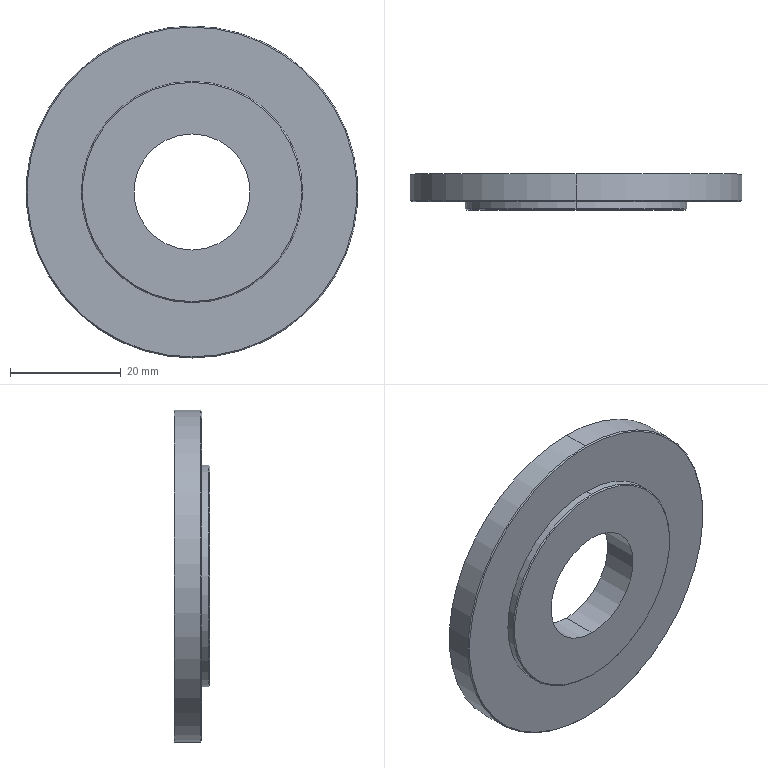Part | STEP file | Guide wheel mechanism revised.sldasm-Part-432 | 1 solid | 25 faces | box 60 x 6.5 x 60 mm | volume 13262 mm3 | cylinder 14 | plane 7 | cone 4 | commonest cylinder face diameters 8 x8 21 x2 40 x2 60 x2
STEP:
#1=CARTESIAN_POINT('',(0.,-1.5,-19.8));
#2=VERTEX_POINT('',#1);
#3=CARTESIAN_POINT('',(0.,-1.5,19.8));
#4=VERTEX_POINT('',#3);
#5=CARTESIAN_POINT('',(0.,-1.5,0.));
#6=DIRECTION('',(0.,-1.,0.));
#7=DIRECTION('',(0.,0.,1.));
#8=AXIS2_PLACEMENT_3D('',#5,#6,#7);
#9=CIRCLE('',#8,19.8);
#10=EDGE_CURVE('',#2,#4,#9,.T.);
#11=ORIENTED_EDGE('',*,*,#10,.F.);
#12=CARTESIAN_POINT('',(0.,-1.3,-20.));
#13=VERTEX_POINT('',#12);
#14=CARTESIAN_POINT('',(0.,-1.3,-20.));
#15=DIRECTION('',(0.,0.7071,-0.7071));
#16=VECTOR('',#15,1000.);
#17=LINE('',#14,#16);
#18=EDGE_CURVE('',#2,#13,#17,.T.);
#19=ORIENTED_EDGE('',*,*,#18,.T.);
#20=CARTESIAN_POINT('',(0.,-1.3,20.));
#21=VERTEX_POINT('',#20);
#22=CARTESIAN_POINT('',(0.,-1.3,0.));
#23=DIRECTION('',(0.,1.,0.));
#24=DIRECTION('',(0.,0.,1.));
#25=AXIS2_PLACEMENT_3D('',#22,#23,#24);
#26=CIRCLE('',#25,20.);
#27=EDGE_CURVE('',#21,#13,#26,.T.);
#28=ORIENTED_EDGE('',*,*,#27,.F.);
#29=CARTESIAN_POINT('',(0.,-1.3,20.));
#30=DIRECTION('',(0.,0.7071,0.7071));
#31=VECTOR('',#30,1000.);
#32=LINE('',#29,#31);
#33=EDGE_CURVE('',#4,#21,#32,.T.);
#34=ORIENTED_EDGE('',*,*,#33,.F.);
#35=EDGE_LOOP('',(#11,#19,#28,#34));
#36=FACE_OUTER_BOUND('',#35,.T.);
#37=CARTESIAN_POINT('',(0.,-1.3,0.));
#38=DIRECTION('',(0.,1.,0.));
#39=DIRECTION('',(0.,0.,1.));
#40=AXIS2_PLACEMENT_3D('',#37,#38,#39);
#41=CONICAL_SURFACE('',#40,20.,0.7854);
#42=ADVANCED_FACE('',(#36),#41,.T.);
#43=CARTESIAN_POINT('',(0.,0.,-29.8));
#44=VERTEX_POINT('',#43);
#45=CARTESIAN_POINT('',(0.,0.,29.8));
#46=VERTEX_POINT('',#45);
#47=CARTESIAN_POINT('',(0.,0.,0.));
#48=DIRECTION('',(0.,-1.,0.));
#49=DIRECTION('',(0.,0.,1.));
#50=AXIS2_PLACEMENT_3D('',#47,#48,#49);
#51=CIRCLE('',#50,29.8);
#52=EDGE_CURVE('',#44,#46,#51,.T.);
#53=ORIENTED_EDGE('',*,*,#52,.F.);
#54=CARTESIAN_POINT('',(0.,0.2,-30.));
#55=VERTEX_POINT('',#54);
#56=CARTESIAN_POINT('',(0.,0.2,-30.));
#57=DIRECTION('',(0.,0.7071,-0.7071));
#58=VECTOR('',#57,1000.);
#59=LINE('',#56,#58);
#60=EDGE_CURVE('',#44,#55,#59,.T.);
#61=ORIENTED_EDGE('',*,*,#60,.T.);
#62=CARTESIAN_POINT('',(0.,0.2,30.));
#63=VERTEX_POINT('',#62);
#64=CARTESIAN_POINT('',(0.,0.2,0.));
#65=DIRECTION('',(0.,1.,0.));
#66=DIRECTION('',(0.,0.,1.));
#67=AXIS2_PLACEMENT_3D('',#64,#65,#66);
#68=CIRCLE('',#67,30.);
#69=EDGE_CURVE('',#63,#55,#68,.T.);
#70=ORIENTED_EDGE('',*,*,#69,.F.);
#71=CARTESIAN_POINT('',(0.,0.2,30.));
#72=DIRECTION('',(0.,0.7071,0.7071));
#73=VECTOR('',#72,1000.);
#74=LINE('',#71,#73);
#75=EDGE_CURVE('',#46,#63,#74,.T.);
#76=ORIENTED_EDGE('',*,*,#75,.F.);
#77=EDGE_LOOP('',(#53,#61,#70,#76));
#78=FACE_OUTER_BOUND('',#77,.T.);
#79=CARTESIAN_POINT('',(0.,0.2,0.));
#80=DIRECTION('',(0.,1.,0.));
#81=DIRECTION('',(0.,0.,1.));
#82=AXIS2_PLACEMENT_3D('',#79,#80,#81);
#83=CONICAL_SURFACE('',#82,30.,0.7854);
#84=ADVANCED_FACE('',(#78),#83,.T.);
#85=ORIENTED_EDGE('',*,*,#27,.T.);
#86=CARTESIAN_POINT('',(0.,0.,-20.));
#87=VERTEX_POINT('',#86);
#88=CARTESIAN_POINT('',(0.,-1.5,-20.));
#89=DIRECTION('',(0.,1.,0.));
#90=VECTOR('',#89,1000.);
#91=LINE('',#88,#90);
#92=EDGE_CURVE('',#13,#87,#91,.T.);
#93=ORIENTED_EDGE('',*,*,#92,.T.);
#94=CARTESIAN_POINT('',(0.,0.,20.));
#95=VERTEX_POINT('',#94);
#96=CARTESIAN_POINT('',(0.,0.,0.));
#97=DIRECTION('',(0.,1.,0.));
#98=DIRECTION('',(0.,0.,1.));
#99=AXIS2_PLACEMENT_3D('',#96,#97,#98);
#100=CIRCLE('',#99,20.);
#101=EDGE_CURVE('',#95,#87,#100,.T.);
#102=ORIENTED_EDGE('',*,*,#101,.F.);
#103=CARTESIAN_POINT('',(0.,-1.5,20.));
#104=DIRECTION('',(0.,1.,0.));
#105=VECTOR('',#104,1000.);
#106=LINE('',#103,#105);
#107=EDGE_CURVE('',#21,#95,#106,.T.);
#108=ORIENTED_EDGE('',*,*,#107,.F.);
#109=EDGE_LOOP('',(#85,#93,#102,#108));
#110=FACE_OUTER_BOUND('',#109,.T.);
#111=CARTESIAN_POINT('',(0.,-1.5,0.));
#112=DIRECTION('',(0.,1.,0.));
#113=DIRECTION('',(0.,0.,1.));
#114=AXIS2_PLACEMENT_3D('',#111,#112,#113);
#115=CYLINDRICAL_SURFACE('',#114,20.);
#116=ADVANCED_FACE('',(#110),#115,.T.);
#117=CARTESIAN_POINT('',(0.,2.5,16.));
#118=VERTEX_POINT('',#117);
#119=CARTESIAN_POINT('',(0.,2.5,24.));
#120=VERTEX_POINT('',#119);
#121=CARTESIAN_POINT('',(0.,2.5,20.));
#122=DIRECTION('',(0.,1.,0.));
#123=DIRECTION('',(0.,0.,1.));
#124=AXIS2_PLACEMENT_3D('',#121,#122,#123);
#125=CIRCLE('',#124,4.);
#126=EDGE_CURVE('',#118,#120,#125,.T.);
#127=ORIENTED_EDGE('',*,*,#126,.F.);
#128=CARTESIAN_POINT('',(0.,5.,16.));
#129=VERTEX_POINT('',#128);
#130=CARTESIAN_POINT('',(0.,2.5,16.));
#131=DIRECTION('',(0.,1.,0.));
#132=VECTOR('',#131,1000.);
#133=LINE('',#130,#132);
#134=EDGE_CURVE('',#118,#129,#133,.T.);
#135=ORIENTED_EDGE('',*,*,#134,.T.);
#136=CARTESIAN_POINT('',(0.,5.,24.));
#137=VERTEX_POINT('',#136);
#138=CARTESIAN_POINT('',(0.,5.,20.));
#139=DIRECTION('',(0.,1.,0.));
#140=DIRECTION('',(0.,0.,1.));
#141=AXIS2_PLACEMENT_3D('',#138,#139,#140);
#142=CIRCLE('',#141,4.);
#143=EDGE_CURVE('',#129,#137,#142,.T.);
#144=ORIENTED_EDGE('',*,*,#143,.T.);
#145=CARTESIAN_POINT('',(0.,2.5,24.));
#146=DIRECTION('',(0.,1.,0.));
#147=VECTOR('',#146,1000.);
#148=LINE('',#145,#147);
#149=EDGE_CURVE('',#120,#137,#148,.T.);
#150=ORIENTED_EDGE('',*,*,#149,.F.);
#151=EDGE_LOOP('',(#127,#135,#144,#150));
#152=FACE_OUTER_BOUND('',#151,.T.);
#153=CARTESIAN_POINT('',(0.,2.5,20.));
#154=DIRECTION('',(0.,1.,0.));
#155=DIRECTION('',(0.,0.,1.));
#156=AXIS2_PLACEMENT_3D('',#153,#154,#155);
#157=CYLINDRICAL_SURFACE('',#156,4.);
#158=ADVANCED_FACE('',(#152),#157,.F.);
#159=CARTESIAN_POINT('',(20.,2.5,-4.));
#160=VERTEX_POINT('',#159);
#161=CARTESIAN_POINT('',(20.,2.5,4.));
#162=VERTEX_POINT('',#161);
#163=CARTESIAN_POINT('',(20.,2.5,0.));
#164=DIRECTION('',(0.,1.,0.));
#165=DIRECTION('',(0.,0.,1.));
#166=AXIS2_PLACEMENT_3D('',#163,#164,#165);
#167=CIRCLE('',#166,4.);
#168=EDGE_CURVE('',#160,#162,#167,.T.);
#169=ORIENTED_EDGE('',*,*,#168,.F.);
#170=CARTESIAN_POINT('',(20.,5.,-4.));
#171=VERTEX_POINT('',#170);
#172=CARTESIAN_POINT('',(20.,2.5,-4.));
#173=DIRECTION('',(0.,1.,0.));
#174=VECTOR('',#173,1000.);
#175=LINE('',#172,#174);
#176=EDGE_CURVE('',#160,#171,#175,.T.);
#177=ORIENTED_EDGE('',*,*,#176,.T.);
#178=CARTESIAN_POINT('',(20.,5.,4.));
#179=VERTEX_POINT('',#178);
#180=CARTESIAN_POINT('',(20.,5.,0.));
#181=DIRECTION('',(0.,1.,0.));
#182=DIRECTION('',(0.,0.,1.));
#183=AXIS2_PLACEMENT_3D('',#180,#181,#182);
#184=CIRCLE('',#183,4.);
#185=EDGE_CURVE('',#171,#179,#184,.T.);
#186=ORIENTED_EDGE('',*,*,#185,.T.);
#187=CARTESIAN_POINT('',(20.,2.5,4.));
#188=DIRECTION('',(0.,1.,0.));
#189=VECTOR('',#188,1000.);
#190=LINE('',#187,#189);
#191=EDGE_CURVE('',#162,#179,#190,.T.);
#192=ORIENTED_EDGE('',*,*,#191,.F.);
#193=EDGE_LOOP('',(#169,#177,#186,#192));
#194=FACE_OUTER_BOUND('',#193,.T.);
#195=CARTESIAN_POINT('',(20.,2.5,0.));
#196=DIRECTION('',(0.,1.,0.));
#197=DIRECTION('',(0.,0.,1.));
#198=AXIS2_PLACEMENT_3D('',#195,#196,#197);
#199=CYLINDRICAL_SURFACE('',#198,4.);
#200=ADVANCED_FACE('',(#194),#199,.F.);
#201=CARTESIAN_POINT('',(-20.,2.5,-4.));
#202=VERTEX_POINT('',#201);
#203=CARTESIAN_POINT('',(-20.,2.5,4.));
#204=VERTEX_POINT('',#203);
#205=CARTESIAN_POINT('',(-20.,2.5,0.));
#206=DIRECTION('',(0.,1.,0.));
#207=DIRECTION('',(0.,0.,1.));
#208=AXIS2_PLACEMENT_3D('',#205,#206,#207);
#209=CIRCLE('',#208,4.);
#210=EDGE_CURVE('',#202,#204,#209,.T.);
#211=ORIENTED_EDGE('',*,*,#210,.F.);
#212=CARTESIAN_POINT('',(-20.,5.,-4.));
#213=VERTEX_POINT('',#212);
#214=CARTESIAN_POINT('',(-20.,2.5,-4.));
#215=DIRECTION('',(0.,1.,0.));
#216=VECTOR('',#215,1000.);
#217=LINE('',#214,#216);
#218=EDGE_CURVE('',#202,#213,#217,.T.);
#219=ORIENTED_EDGE('',*,*,#218,.T.);
#220=CARTESIAN_POINT('',(-20.,5.,4.));
#221=VERTEX_POINT('',#220);
#222=CARTESIAN_POINT('',(-20.,5.,0.));
#223=DIRECTION('',(0.,1.,0.));
#224=DIRECTION('',(0.,0.,1.));
#225=AXIS2_PLACEMENT_3D('',#222,#223,#224);
#226=CIRCLE('',#225,4.);
#227=EDGE_CURVE('',#213,#221,#226,.T.);
#228=ORIENTED_EDGE('',*,*,#227,.T.);
#229=CARTESIAN_POINT('',(-20.,2.5,4.));
#230=DIRECTION('',(0.,1.,0.));
#231=VECTOR('',#230,1000.);
#232=LINE('',#229,#231);
#233=EDGE_CURVE('',#204,#221,#232,.T.);
#234=ORIENTED_EDGE('',*,*,#233,.F.);
#235=EDGE_LOOP('',(#211,#219,#228,#234));
#236=FACE_OUTER_BOUND('',#235,.T.);
#237=CARTESIAN_POINT('',(-20.,2.5,0.));
#238=DIRECTION('',(0.,1.,0.));
#239=DIRECTION('',(0.,0.,1.));
#240=AXIS2_PLACEMENT_3D('',#237,#238,#239);
#241=CYLINDRICAL_SURFACE('',#240,4.);
#242=ADVANCED_FACE('',(#236),#241,.F.);
#243=CARTESIAN_POINT('',(0.,2.5,-24.));
#244=VERTEX_POINT('',#243);
#245=CARTESIAN_POINT('',(0.,2.5,-16.));
#246=VERTEX_POINT('',#245);
#247=CARTESIAN_POINT('',(0.,2.5,-20.));
#248=DIRECTION('',(0.,1.,0.));
#249=DIRECTION('',(0.,0.,1.));
#250=AXIS2_PLACEMENT_3D('',#247,#248,#249);
#251=CIRCLE('',#250,4.);
#252=EDGE_CURVE('',#244,#246,#251,.T.);
#253=ORIENTED_EDGE('',*,*,#252,.F.);
#254=CARTESIAN_POINT('',(0.,5.,-24.));
#255=VERTEX_POINT('',#254);
#256=CARTESIAN_POINT('',(0.,2.5,-24.));
#257=DIRECTION('',(0.,1.,0.));
#258=VECTOR('',#257,1000.);
#259=LINE('',#256,#258);
#260=EDGE_CURVE('',#244,#255,#259,.T.);
#261=ORIENTED_EDGE('',*,*,#260,.T.);
#262=CARTESIAN_POINT('',(0.,5.,-16.));
#263=VERTEX_POINT('',#262);
#264=CARTESIAN_POINT('',(0.,5.,-20.));
#265=DIRECTION('',(0.,1.,0.));
#266=DIRECTION('',(0.,0.,1.));
#267=AXIS2_PLACEMENT_3D('',#264,#265,#266);
#268=CIRCLE('',#267,4.);
#269=EDGE_CURVE('',#255,#263,#268,.T.);
#270=ORIENTED_EDGE('',*,*,#269,.T.);
#271=CARTESIAN_POINT('',(0.,2.5,-16.));
#272=DIRECTION('',(0.,1.,0.));
#273=VECTOR('',#272,1000.);
#274=LINE('',#271,#273);
#275=EDGE_CURVE('',#246,#263,#274,.T.);
#276=ORIENTED_EDGE('',*,*,#275,.F.);
#277=EDGE_LOOP('',(#253,#261,#270,#276));
#278=FACE_OUTER_BOUND('',#277,.T.);
#279=CARTESIAN_POINT('',(0.,2.5,-20.));
#280=DIRECTION('',(0.,1.,0.));
#281=DIRECTION('',(0.,0.,1.));
#282=AXIS2_PLACEMENT_3D('',#279,#280,#281);
#283=CYLINDRICAL_SURFACE('',#282,4.);
#284=ADVANCED_FACE('',(#278),#283,.F.);
#285=CARTESIAN_POINT('',(0.,5.,-10.5));
#286=VERTEX_POINT('',#285);
#287=CARTESIAN_POINT('',(0.,5.,10.5));
#288=VERTEX_POINT('',#287);
#289=CARTESIAN_POINT('',(0.,5.,0.));
#290=DIRECTION('',(0.,1.,0.));
#291=DIRECTION('',(0.,0.,1.));
#292=AXIS2_PLACEMENT_3D('',#289,#290,#291);
#293=CIRCLE('',#292,10.5);
#294=EDGE_CURVE('',#286,#288,#293,.T.);
#295=ORIENTED_EDGE('',*,*,#294,.T.);
#296=CARTESIAN_POINT('',(0.,-1.5,10.5));
#297=VERTEX_POINT('',#296);
#298=CARTESIAN_POINT('',(0.,5.,10.5));
#299=DIRECTION('',(0.,-1.,0.));
#300=VECTOR('',#299,1000.);
#301=LINE('',#298,#300);
#302=EDGE_CURVE('',#288,#297,#301,.T.);
#303=ORIENTED_EDGE('',*,*,#302,.T.);
#304=CARTESIAN_POINT('',(0.,-1.5,-10.5));
#305=VERTEX_POINT('',#304);
#306=CARTESIAN_POINT('',(0.,-1.5,0.));
#307=DIRECTION('',(0.,1.,0.));
#308=DIRECTION('',(0.,0.,1.));
#309=AXIS2_PLACEMENT_3D('',#306,#307,#308);
#310=CIRCLE('',#309,10.5);
#311=EDGE_CURVE('',#305,#297,#310,.T.);
#312=ORIENTED_EDGE('',*,*,#311,.F.);
#313=CARTESIAN_POINT('',(0.,5.,-10.5));
#314=DIRECTION('',(0.,-1.,0.));
#315=VECTOR('',#314,1000.);
#316=LINE('',#313,#315);
#317=EDGE_CURVE('',#286,#305,#316,.T.);
#318=ORIENTED_EDGE('',*,*,#317,.F.);
#319=EDGE_LOOP('',(#295,#303,#312,#318));
#320=FACE_OUTER_BOUND('',#319,.T.);
#321=CARTESIAN_POINT('',(0.,5.,0.));
#322=DIRECTION('',(0.,-1.,0.));
#323=DIRECTION('',(0.,0.,-1.));
#324=AXIS2_PLACEMENT_3D('',#321,#322,#323);
#325=CYLINDRICAL_SURFACE('',#324,10.5);
#326=ADVANCED_FACE('',(#320),#325,.F.);
#327=CARTESIAN_POINT('',(0.,5.,30.));
#328=VERTEX_POINT('',#327);
#329=CARTESIAN_POINT('',(0.,5.,-30.));
#330=VERTEX_POINT('',#329);
#331=CARTESIAN_POINT('',(0.,5.,0.));
#332=DIRECTION('',(0.,1.,0.));
#333=DIRECTION('',(0.,0.,1.));
#334=AXIS2_PLACEMENT_3D('',#331,#332,#333);
#335=CIRCLE('',#334,30.);
#336=EDGE_CURVE('',#328,#330,#335,.T.);
#337=ORIENTED_EDGE('',*,*,#336,.F.);
#338=CARTESIAN_POINT('',(0.,5.,30.));
#339=DIRECTION('',(0.,-1.,0.));
#340=VECTOR('',#339,1000.);
#341=LINE('',#338,#340);
#342=EDGE_CURVE('',#328,#63,#341,.T.);
#343=ORIENTED_EDGE('',*,*,#342,.T.);
#344=ORIENTED_EDGE('',*,*,#69,.T.);
#345=CARTESIAN_POINT('',(0.,5.,-30.));
#346=DIRECTION('',(0.,-1.,0.));
#347=VECTOR('',#346,1000.);
#348=LINE('',#345,#347);
#349=EDGE_CURVE('',#330,#55,#348,.T.);
#350=ORIENTED_EDGE('',*,*,#349,.F.);
#351=EDGE_LOOP('',(#337,#343,#344,#350));
#352=FACE_OUTER_BOUND('',#351,.T.);
#353=CARTESIAN_POINT('',(0.,5.,0.));
#354=DIRECTION('',(0.,-1.,0.));
#355=DIRECTION('',(0.,0.,-1.));
#356=AXIS2_PLACEMENT_3D('',#353,#354,#355);
#357=CYLINDRICAL_SURFACE('',#356,30.);
#358=ADVANCED_FACE('',(#352),#357,.T.);
#359=CARTESIAN_POINT('',(0.,5.,20.));
#360=DIRECTION('',(0.,1.,0.));
#361=DIRECTION('',(0.,0.,1.));
#362=AXIS2_PLACEMENT_3D('',#359,#360,#361);
#363=CIRCLE('',#362,4.);
#364=EDGE_CURVE('',#137,#129,#363,.T.);
#365=ORIENTED_EDGE('',*,*,#364,.F.);
#366=ORIENTED_EDGE('',*,*,#143,.F.);
#367=EDGE_LOOP('',(#365,#366));
#368=FACE_BOUND('',#367,.T.);
#369=CARTESIAN_POINT('',(20.,5.,0.));
#370=DIRECTION('',(0.,1.,0.));
#371=DIRECTION('',(0.,0.,1.));
#372=AXIS2_PLACEMENT_3D('',#369,#370,#371);
#373=CIRCLE('',#372,4.);
#374=EDGE_CURVE('',#179,#171,#373,.T.);
#375=ORIENTED_EDGE('',*,*,#374,.F.);
#376=ORIENTED_EDGE('',*,*,#185,.F.);
#377=EDGE_LOOP('',(#375,#376));
#378=FACE_BOUND('',#377,.T.);
#379=CARTESIAN_POINT('',(-20.,5.,0.));
#380=DIRECTION('',(0.,1.,0.));
#381=DIRECTION('',(0.,0.,1.));
#382=AXIS2_PLACEMENT_3D('',#379,#380,#381);
#383=CIRCLE('',#382,4.);
#384=EDGE_CURVE('',#221,#213,#383,.T.);
#385=ORIENTED_EDGE('',*,*,#384,.F.);
#386=ORIENTED_EDGE('',*,*,#227,.F.);
#387=EDGE_LOOP('',(#385,#386));
#388=FACE_BOUND('',#387,.T.);
#389=CARTESIAN_POINT('',(0.,5.,-20.));
#390=DIRECTION('',(0.,1.,0.));
#391=DIRECTION('',(0.,0.,1.));
#392=AXIS2_PLACEMENT_3D('',#389,#390,#391);
#393=CIRCLE('',#392,4.);
#394=EDGE_CURVE('',#263,#255,#393,.T.);
#395=ORIENTED_EDGE('',*,*,#394,.F.);
#396=ORIENTED_EDGE('',*,*,#269,.F.);
#397=EDGE_LOOP('',(#395,#396));
#398=FACE_BOUND('',#397,.T.);
#399=CARTESIAN_POINT('',(0.,5.,0.));
#400=DIRECTION('',(0.,1.,0.));
#401=DIRECTION('',(0.,0.,1.));
#402=AXIS2_PLACEMENT_3D('',#399,#400,#401);
#403=CIRCLE('',#402,30.);
#404=EDGE_CURVE('',#330,#328,#403,.T.);
#405=ORIENTED_EDGE('',*,*,#404,.T.);
#406=ORIENTED_EDGE('',*,*,#336,.T.);
#407=EDGE_LOOP('',(#405,#406));
#408=FACE_OUTER_BOUND('',#407,.T.);
#409=ORIENTED_EDGE('',*,*,#294,.F.);
#410=CARTESIAN_POINT('',(0.,5.,0.));
#411=DIRECTION('',(0.,1.,0.));
#412=DIRECTION('',(0.,0.,1.));
#413=AXIS2_PLACEMENT_3D('',#410,#411,#412);
#414=CIRCLE('',#413,10.5);
#415=EDGE_CURVE('',#288,#286,#414,.T.);
#416=ORIENTED_EDGE('',*,*,#415,.F.);
#417=EDGE_LOOP('',(#409,#416));
#418=FACE_BOUND('',#417,.T.);
#419=CARTESIAN_POINT('',(0.,5.,0.));
#420=DIRECTION('',(0.,1.,0.));
#421=DIRECTION('',(0.,0.,1.));
#422=AXIS2_PLACEMENT_3D('',#419,#420,#421);
#423=PLANE('',#422);
#424=ADVANCED_FACE('',(#368,#378,#388,#398,#408,#418),#423,.T.);
#425=CARTESIAN_POINT('',(0.,0.,0.));
#426=DIRECTION('',(0.,-1.,0.));
#427=DIRECTION('',(0.,0.,1.));
#428=AXIS2_PLACEMENT_3D('',#425,#426,#427);
#429=CIRCLE('',#428,29.8);
#430=EDGE_CURVE('',#46,#44,#429,.T.);
#431=ORIENTED_EDGE('',*,*,#430,.T.);
#432=ORIENTED_EDGE('',*,*,#52,.T.);
#433=EDGE_LOOP('',(#431,#432));
#434=FACE_OUTER_BOUND('',#433,.T.);
#435=ORIENTED_EDGE('',*,*,#101,.T.);
#436=CARTESIAN_POINT('',(0.,0.,0.));
#437=DIRECTION('',(0.,1.,0.));
#438=DIRECTION('',(0.,0.,1.));
#439=AXIS2_PLACEMENT_3D('',#436,#437,#438);
#440=CIRCLE('',#439,20.);
#441=EDGE_CURVE('',#87,#95,#440,.T.);
#442=ORIENTED_EDGE('',*,*,#441,.T.);
#443=EDGE_LOOP('',(#435,#442));
#444=FACE_BOUND('',#443,.T.);
#445=CARTESIAN_POINT('',(0.,0.,0.));
#446=DIRECTION('',(0.,1.,0.));
#447=DIRECTION('',(0.,0.,1.));
#448=AXIS2_PLACEMENT_3D('',#445,#446,#447);
#449=PLANE('',#448);
#450=ADVANCED_FACE('',(#434,#444),#449,.F.);
#451=ORIENTED_EDGE('',*,*,#342,.F.);
#452=ORIENTED_EDGE('',*,*,#404,.F.);
#453=ORIENTED_EDGE('',*,*,#349,.T.);
#454=CARTESIAN_POINT('',(0.,0.2,0.));
#455=DIRECTION('',(0.,1.,0.));
#456=DIRECTION('',(0.,0.,1.));
#457=AXIS2_PLACEMENT_3D('',#454,#455,#456);
#458=CIRCLE('',#457,30.);
#459=EDGE_CURVE('',#55,#63,#458,.T.);
#460=ORIENTED_EDGE('',*,*,#459,.T.);
#461=EDGE_LOOP('',(#451,#452,#453,#460));
#462=FACE_OUTER_BOUND('',#461,.T.);
#463=CARTESIAN_POINT('',(0.,5.,0.));
#464=DIRECTION('',(0.,-1.,0.));
#465=DIRECTION('',(0.,0.,-1.));
#466=AXIS2_PLACEMENT_3D('',#463,#464,#465);
#467=CYLINDRICAL_SURFACE('',#466,30.);
#468=ADVANCED_FACE('',(#462),#467,.T.);
#469=ORIENTED_EDGE('',*,*,#302,.F.);
#470=ORIENTED_EDGE('',*,*,#415,.T.);
#471=ORIENTED_EDGE('',*,*,#317,.T.);
#472=CARTESIAN_POINT('',(0.,-1.5,0.));
#473=DIRECTION('',(0.,1.,0.));
#474=DIRECTION('',(0.,0.,1.));
#475=AXIS2_PLACEMENT_3D('',#472,#473,#474);
#476=CIRCLE('',#475,10.5);
#477=EDGE_CURVE('',#297,#305,#476,.T.);
#478=ORIENTED_EDGE('',*,*,#477,.F.);
#479=EDGE_LOOP('',(#469,#470,#471,#478));
#480=FACE_OUTER_BOUND('',#479,.T.);
#481=CARTESIAN_POINT('',(0.,5.,0.));
#482=DIRECTION('',(0.,-1.,0.));
#483=DIRECTION('',(0.,0.,-1.));
#484=AXIS2_PLACEMENT_3D('',#481,#482,#483);
#485=CYLINDRICAL_SURFACE('',#484,10.5);
#486=ADVANCED_FACE('',(#480),#485,.F.);
#487=ORIENTED_EDGE('',*,*,#260,.F.);
#488=CARTESIAN_POINT('',(0.,2.5,-20.));
#489=DIRECTION('',(0.,1.,0.));
#490=DIRECTION('',(0.,0.,1.));
#491=AXIS2_PLACEMENT_3D('',#488,#489,#490);
#492=CIRCLE('',#491,4.);
#493=EDGE_CURVE('',#246,#244,#492,.T.);
#494=ORIENTED_EDGE('',*,*,#493,.F.);
#495=ORIENTED_EDGE('',*,*,#275,.T.);
#496=ORIENTED_EDGE('',*,*,#394,.T.);
#497=EDGE_LOOP('',(#487,#494,#495,#496));
#498=FACE_OUTER_BOUND('',#497,.T.);
#499=CARTESIAN_POINT('',(0.,2.5,-20.));
#500=DIRECTION('',(0.,1.,0.));
#501=DIRECTION('',(0.,0.,1.));
#502=AXIS2_PLACEMENT_3D('',#499,#500,#501);
#503=CYLINDRICAL_SURFACE('',#502,4.);
#504=ADVANCED_FACE('',(#498),#503,.F.);
#505=ORIENTED_EDGE('',*,*,#493,.T.);
#506=ORIENTED_EDGE('',*,*,#252,.T.);
#507=EDGE_LOOP('',(#505,#506));
#508=FACE_OUTER_BOUND('',#507,.T.);
#509=CARTESIAN_POINT('',(0.,2.5,-20.));
#510=DIRECTION('',(0.,1.,0.));
#511=DIRECTION('',(0.,0.,1.));
#512=AXIS2_PLACEMENT_3D('',#509,#510,#511);
#513=PLANE('',#512);
#514=ADVANCED_FACE('',(#508),#513,.T.);
#515=ORIENTED_EDGE('',*,*,#218,.F.);
#516=CARTESIAN_POINT('',(-20.,2.5,0.));
#517=DIRECTION('',(0.,1.,0.));
#518=DIRECTION('',(0.,0.,1.));
#519=AXIS2_PLACEMENT_3D('',#516,#517,#518);
#520=CIRCLE('',#519,4.);
#521=EDGE_CURVE('',#204,#202,#520,.T.);
#522=ORIENTED_EDGE('',*,*,#521,.F.);
#523=ORIENTED_EDGE('',*,*,#233,.T.);
#524=ORIENTED_EDGE('',*,*,#384,.T.);
#525=EDGE_LOOP('',(#515,#522,#523,#524));
#526=FACE_OUTER_BOUND('',#525,.T.);
#527=CARTESIAN_POINT('',(-20.,2.5,0.));
#528=DIRECTION('',(0.,1.,0.));
#529=DIRECTION('',(0.,0.,1.));
#530=AXIS2_PLACEMENT_3D('',#527,#528,#529);
#531=CYLINDRICAL_SURFACE('',#530,4.);
#532=ADVANCED_FACE('',(#526),#531,.F.);
#533=ORIENTED_EDGE('',*,*,#521,.T.);
#534=ORIENTED_EDGE('',*,*,#210,.T.);
#535=EDGE_LOOP('',(#533,#534));
#536=FACE_OUTER_BOUND('',#535,.T.);
#537=CARTESIAN_POINT('',(-20.,2.5,0.));
#538=DIRECTION('',(0.,1.,0.));
#539=DIRECTION('',(0.,0.,1.));
#540=AXIS2_PLACEMENT_3D('',#537,#538,#539);
#541=PLANE('',#540);
#542=ADVANCED_FACE('',(#536),#541,.T.);
#543=ORIENTED_EDGE('',*,*,#176,.F.);
#544=CARTESIAN_POINT('',(20.,2.5,0.));
#545=DIRECTION('',(0.,1.,0.));
#546=DIRECTION('',(0.,0.,1.));
#547=AXIS2_PLACEMENT_3D('',#544,#545,#546);
#548=CIRCLE('',#547,4.);
#549=EDGE_CURVE('',#162,#160,#548,.T.);
#550=ORIENTED_EDGE('',*,*,#549,.F.);
#551=ORIENTED_EDGE('',*,*,#191,.T.);
#552=ORIENTED_EDGE('',*,*,#374,.T.);
#553=EDGE_LOOP('',(#543,#550,#551,#552));
#554=FACE_OUTER_BOUND('',#553,.T.);
#555=CARTESIAN_POINT('',(20.,2.5,0.));
#556=DIRECTION('',(0.,1.,0.));
#557=DIRECTION('',(0.,0.,1.));
#558=AXIS2_PLACEMENT_3D('',#555,#556,#557);
#559=CYLINDRICAL_SURFACE('',#558,4.);
#560=ADVANCED_FACE('',(#554),#559,.F.);
#561=ORIENTED_EDGE('',*,*,#549,.T.);
#562=ORIENTED_EDGE('',*,*,#168,.T.);
#563=EDGE_LOOP('',(#561,#562));
#564=FACE_OUTER_BOUND('',#563,.T.);
#565=CARTESIAN_POINT('',(20.,2.5,0.));
#566=DIRECTION('',(0.,1.,0.));
#567=DIRECTION('',(0.,0.,1.));
#568=AXIS2_PLACEMENT_3D('',#565,#566,#567);
#569=PLANE('',#568);
#570=ADVANCED_FACE('',(#564),#569,.T.);
#571=ORIENTED_EDGE('',*,*,#134,.F.);
#572=CARTESIAN_POINT('',(0.,2.5,20.));
#573=DIRECTION('',(0.,1.,0.));
#574=DIRECTION('',(0.,0.,1.));
#575=AXIS2_PLACEMENT_3D('',#572,#573,#574);
#576=CIRCLE('',#575,4.);
#577=EDGE_CURVE('',#120,#118,#576,.T.);
#578=ORIENTED_EDGE('',*,*,#577,.F.);
#579=ORIENTED_EDGE('',*,*,#149,.T.);
#580=ORIENTED_EDGE('',*,*,#364,.T.);
#581=EDGE_LOOP('',(#571,#578,#579,#580));
#582=FACE_OUTER_BOUND('',#581,.T.);
#583=CARTESIAN_POINT('',(0.,2.5,20.));
#584=DIRECTION('',(0.,1.,0.));
#585=DIRECTION('',(0.,0.,1.));
#586=AXIS2_PLACEMENT_3D('',#583,#584,#585);
#587=CYLINDRICAL_SURFACE('',#586,4.);
#588=ADVANCED_FACE('',(#582),#587,.F.);
#589=ORIENTED_EDGE('',*,*,#577,.T.);
#590=ORIENTED_EDGE('',*,*,#126,.T.);
#591=EDGE_LOOP('',(#589,#590));
#592=FACE_OUTER_BOUND('',#591,.T.);
#593=CARTESIAN_POINT('',(0.,2.5,20.));
#594=DIRECTION('',(0.,1.,0.));
#595=DIRECTION('',(0.,0.,1.));
#596=AXIS2_PLACEMENT_3D('',#593,#594,#595);
#597=PLANE('',#596);
#598=ADVANCED_FACE('',(#592),#597,.T.);
#599=ORIENTED_EDGE('',*,*,#92,.F.);
#600=CARTESIAN_POINT('',(0.,-1.3,0.));
#601=DIRECTION('',(0.,1.,0.));
#602=DIRECTION('',(0.,0.,1.));
#603=AXIS2_PLACEMENT_3D('',#600,#601,#602);
#604=CIRCLE('',#603,20.);
#605=EDGE_CURVE('',#13,#21,#604,.T.);
#606=ORIENTED_EDGE('',*,*,#605,.T.);
#607=ORIENTED_EDGE('',*,*,#107,.T.);
#608=ORIENTED_EDGE('',*,*,#441,.F.);
#609=EDGE_LOOP('',(#599,#606,#607,#608));
#610=FACE_OUTER_BOUND('',#609,.T.);
#611=CARTESIAN_POINT('',(0.,-1.5,0.));
#612=DIRECTION('',(0.,1.,0.));
#613=DIRECTION('',(0.,0.,1.));
#614=AXIS2_PLACEMENT_3D('',#611,#612,#613);
#615=CYLINDRICAL_SURFACE('',#614,20.);
#616=ADVANCED_FACE('',(#610),#615,.T.);
#617=CARTESIAN_POINT('',(0.,-1.5,0.));
#618=DIRECTION('',(0.,-1.,0.));
#619=DIRECTION('',(0.,0.,1.));
#620=AXIS2_PLACEMENT_3D('',#617,#618,#619);
#621=CIRCLE('',#620,19.8);
#622=EDGE_CURVE('',#4,#2,#621,.T.);
#623=ORIENTED_EDGE('',*,*,#622,.T.);
#624=ORIENTED_EDGE('',*,*,#10,.T.);
#625=EDGE_LOOP('',(#623,#624));
#626=FACE_OUTER_BOUND('',#625,.T.);
#627=ORIENTED_EDGE('',*,*,#311,.T.);
#628=ORIENTED_EDGE('',*,*,#477,.T.);
#629=EDGE_LOOP('',(#627,#628));
#630=FACE_BOUND('',#629,.T.);
#631=CARTESIAN_POINT('',(0.,-1.5,0.));
#632=DIRECTION('',(0.,1.,0.));
#633=DIRECTION('',(0.,0.,1.));
#634=AXIS2_PLACEMENT_3D('',#631,#632,#633);
#635=PLANE('',#634);
#636=ADVANCED_FACE('',(#626,#630),#635,.F.);
#637=ORIENTED_EDGE('',*,*,#60,.F.);
#638=ORIENTED_EDGE('',*,*,#430,.F.);
#639=ORIENTED_EDGE('',*,*,#75,.T.);
#640=ORIENTED_EDGE('',*,*,#459,.F.);
#641=EDGE_LOOP('',(#637,#638,#639,#640));
#642=FACE_OUTER_BOUND('',#641,.T.);
#643=CARTESIAN_POINT('',(0.,0.2,0.));
#644=DIRECTION('',(0.,1.,0.));
#645=DIRECTION('',(0.,0.,1.));
#646=AXIS2_PLACEMENT_3D('',#643,#644,#645);
#647=CONICAL_SURFACE('',#646,30.,0.7854);
#648=ADVANCED_FACE('',(#642),#647,.T.);
#649=ORIENTED_EDGE('',*,*,#18,.F.);
#650=ORIENTED_EDGE('',*,*,#622,.F.);
#651=ORIENTED_EDGE('',*,*,#33,.T.);
#652=ORIENTED_EDGE('',*,*,#605,.F.);
#653=EDGE_LOOP('',(#649,#650,#651,#652));
#654=FACE_OUTER_BOUND('',#653,.T.);
#655=CARTESIAN_POINT('',(0.,-1.3,0.));
#656=DIRECTION('',(0.,1.,0.));
#657=DIRECTION('',(0.,0.,1.));
#658=AXIS2_PLACEMENT_3D('',#655,#656,#657);
#659=CONICAL_SURFACE('',#658,20.,0.7854);
#660=ADVANCED_FACE('',(#654),#659,.T.);
#661=CLOSED_SHELL('',(#42,#84,#116,#158,#200,#242,#284,#326,#358,#424,#450,#468,#486,#504,#514,#532,#542,#560,#570,#588,#598,#616,#636,#648,#660));
#662=MANIFOLD_SOLID_BREP('',#661);
#663=CARTESIAN_POINT('',(0.,0.,0.));
#664=DIRECTION('',(0.,0.,1.));
#665=DIRECTION('',(1.,0.,0.));
#666=AXIS2_PLACEMENT_3D('',#663,#664,#665);
#667=(LENGTH_UNIT()NAMED_UNIT(*)SI_UNIT(.MILLI.,.METRE.));
#668=UNCERTAINTY_MEASURE_WITH_UNIT(LENGTH_MEASURE(0.00001),#667,'','');
#669=(NAMED_UNIT(*)PLANE_ANGLE_UNIT()SI_UNIT($,.RADIAN.));
#670=(NAMED_UNIT(*)SI_UNIT($,.STERADIAN.)SOLID_ANGLE_UNIT());
#671=(GEOMETRIC_REPRESENTATION_CONTEXT(3)GLOBAL_UNCERTAINTY_ASSIGNED_CONTEXT((#668))GLOBAL_UNIT_ASSIGNED_CONTEXT((#667,#669,#670))REPRESENTATION_CONTEXT('',''));
#672=ADVANCED_BREP_SHAPE_REPRESENTATION('',(#662,#666),#671);